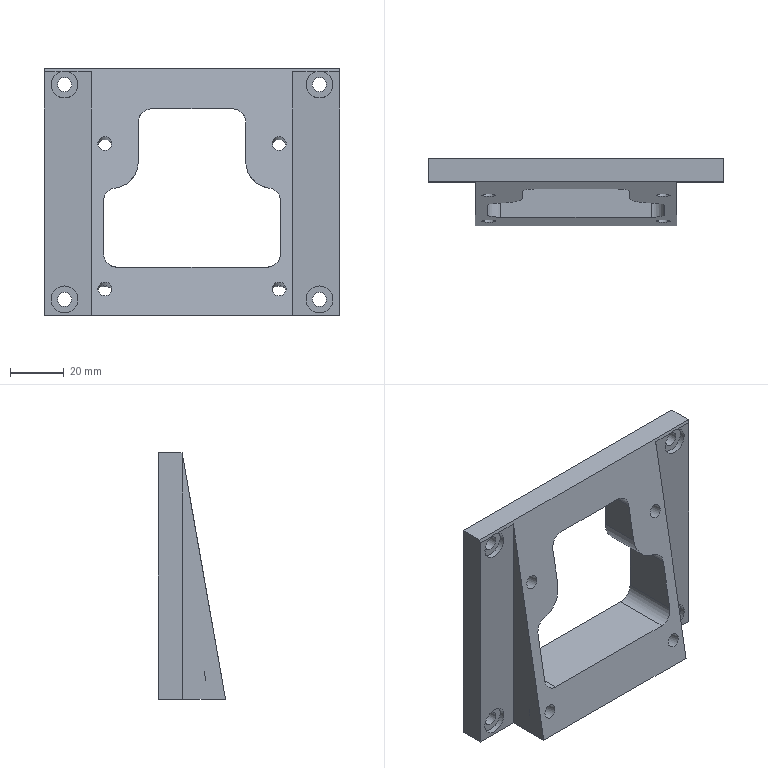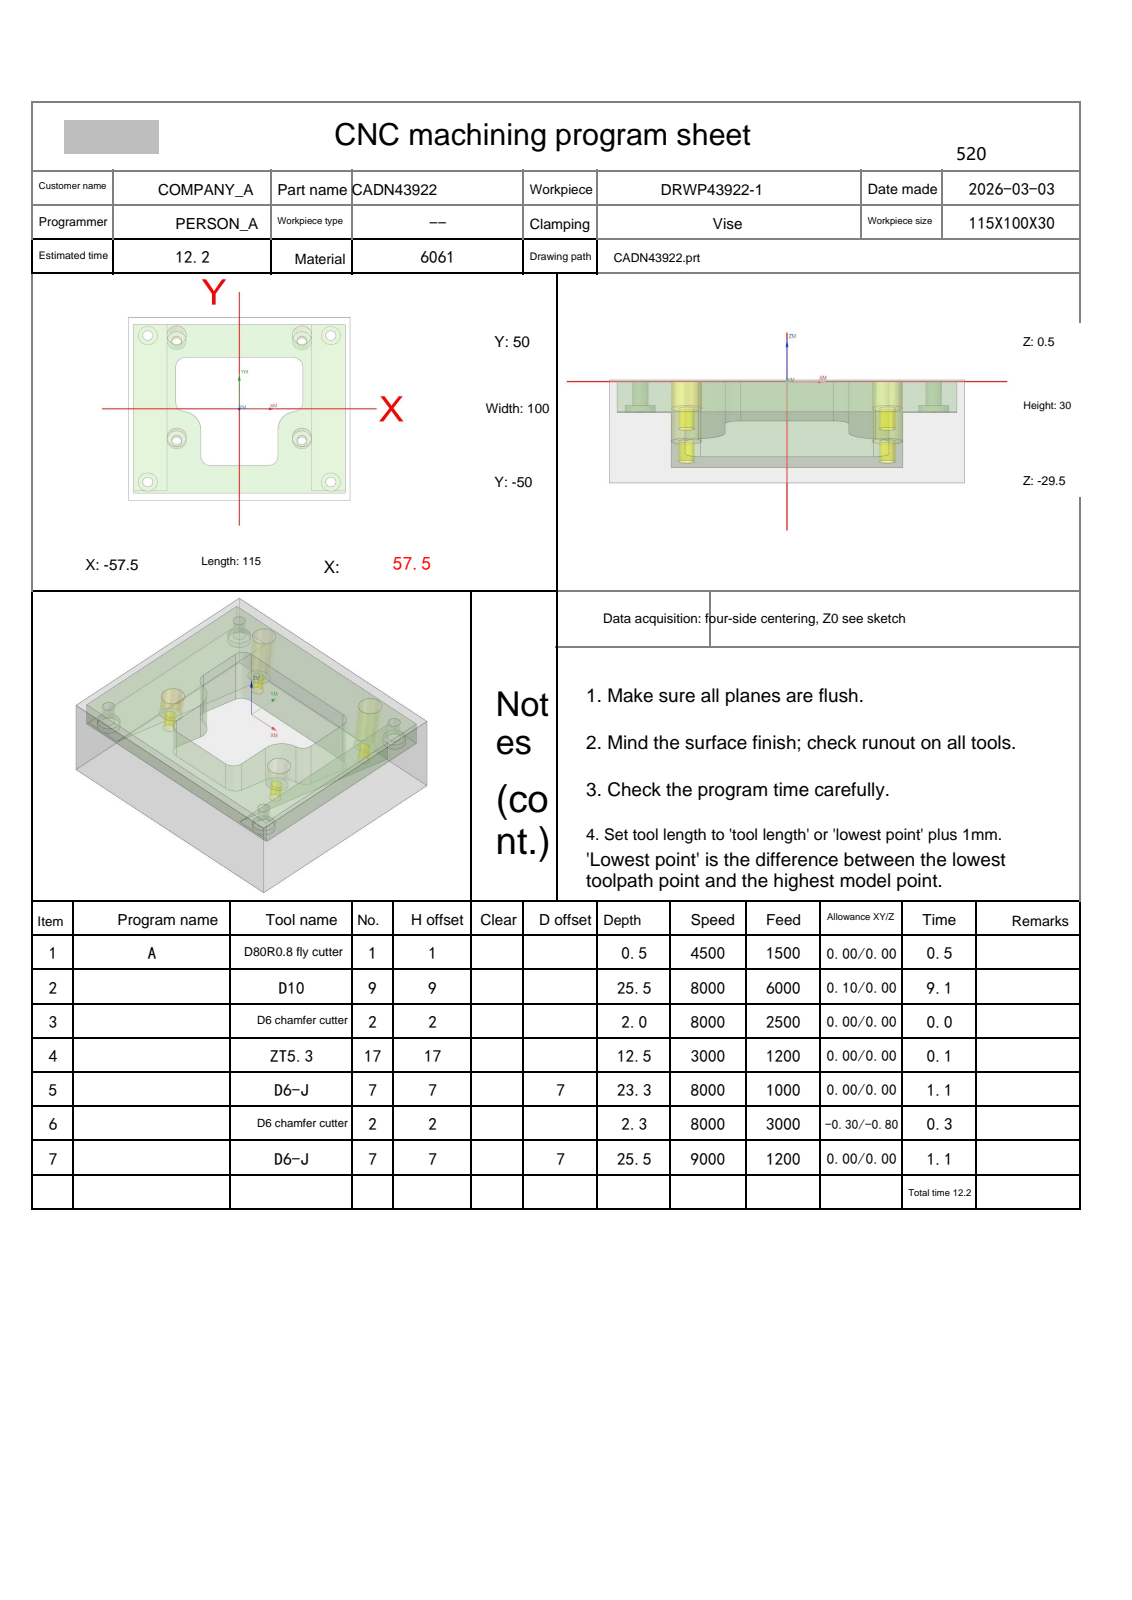NC program | NX | posted by the shop | part box 110 x 25 x 92 mm
Lines 4267 to 4607 of 4607:
N3 T02 M06
(D6 chamfer cutter  D=6. R=0. H=02 ce=0.00 di=0.10)
G00 G90 G54 X47.5 Y40. M03 S8000
G43 H02 Z50.
M08
G98 G81 X47.5 Y40. Z-1.5 R1. F2500.
Y-40.
X-47.5
Y40.
G80
G00 Z50.
G91 G28 Z0.0
M05
M09
G91 G28 Z0.0
M01
N4 T17 M06
(ZT5.3 D=5.3 DR_a=118 H=17)
G00 G90 G54 X47.5 Y40. M03 S3000
G43 H17 Z50.
M08
G98 G83 X47.5 Y40. Z-12. R1. F1200. Q1.5
Y-40.
X-47.5
Y40.
G80
G00 Z50.
G91 G28 Z0.0
M05
M09
G91 G28 Z0.0
M01
N5 T07 M06
(D6-J  D=6. R=0. H=07 ce=0.00 di=0.00)
G00 G90 G54 X29. Y22.801 M03 S8000
G43 H07 Z50.
M08
Z-4.065
G01 Z-4.565 F1000.
G41 D07
Y24.
G03 X28. Y25. I-1. J0.0
G01 X-28.
G03 X-30. Y23. I0.0 J-2.
G01 Y3.5
G03 X-28.267 Y1.518 I2. J0.0
G02 X-17. Y-11.366 I-1.733 J-12.884
G01 Y-26.
G03 X-15. Y-28. I2. J0.0
G01 X15.
G03 X17. Y-26. I0.0 J2.
G01 Y-11.366
G02 X28.267 Y1.518 I13. J0.0
G03 X30. Y3.5 I-.267 J1.982
G01 Y23.
G03 X28. Y25. I-2. J0.0
G01 X27.5
G03 X26.5 Y24. I0.0 J-1.
G01 G40 Y23.8
Z-4.065
G00 X29. Y22.801
Z-8.63
G01 Z-9.13
G41 D07
Y24.
G03 X28. Y25. I-1. J0.0
G01 X-28.
G03 X-30. Y23. I0.0 J-2.
G01 Y3.5
G03 X-28.267 Y1.518 I2. J0.0
G02 X-17. Y-11.366 I-1.733 J-12.884
G01 Y-26.
G03 X-15. Y-28. I2. J0.0
G01 X15.
G03 X17. Y-26. I0.0 J2.
G01 Y-11.366
G02 X28.267 Y1.518 I13. J0.0
G03 X30. Y3.5 I-.267 J1.982
G01 Y23.
G03 X28. Y25. I-2. J0.0
G01 X27.5
G03 X26.5 Y24. I0.0 J-1.
G01 G40 Y23.8
Z-8.63
G00 X29.
Z-13.196
G01 Z-13.696
G41 D07
Y24.
G03 X28. Y25. I-1. J0.0
G01 X-28.
G03 X-30. Y23. I0.0 J-2.
G01 Y3.5
G03 X-28.267 Y1.518 I2. J0.0
G02 X-17. Y-11.366 I-1.733 J-12.884
G01 Y-26.
G03 X-15. Y-28. I2. J0.0
G01 X15.
G03 X17. Y-26. I0.0 J2.
G01 Y-11.366
G02 X28.267 Y1.518 I13. J0.0
G03 X30. Y3.5 I-.267 J1.982
G01 Y23.
G03 X28. Y25. I-2. J0.0
G01 X27.5
G03 X26.5 Y24. I0.0 J-1.
G01 G40 Y23.8
Z-13.196
G00 X29. Y22.801
Z-17.761
G01 Z-18.261
G41 D07
Y24.
G03 X28. Y25. I-1. J0.0
G01 X-28.
G03 X-30. Y23. I0.0 J-2.
G01 Y3.5
G03 X-28.267 Y1.518 I2. J0.0
G02 X-17. Y-11.366 I-1.733 J-12.884
G01 Y-26.
G03 X-15. Y-28. I2. J0.0
G01 X15.
G03 X17. Y-26. I0.0 J2.
G01 Y-11.366
G02 X28.267 Y1.518 I13. J0.0
G03 X30. Y3.5 I-.267 J1.982
G01 Y23.
G03 X28. Y25. I-2. J0.0
G01 X27.5
G03 X26.5 Y24. I0.0 J-1.
G01 G40 Y23.8
Z-17.761
G00 X29. Y22.801
Z-22.326
G01 Z-22.826
G41 D07
Y24.
G03 X28. Y25. I-1. J0.0
G01 X-28.
G03 X-30. Y23. I0.0 J-2.
G01 Y3.5
G03 X-28.267 Y1.518 I2. J0.0
G02 X-17. Y-11.366 I-1.733 J-12.884
G01 Y-26.
G03 X-15. Y-28. I2. J0.0
G01 X15.
G03 X17. Y-26. I0.0 J2.
G01 Y-11.366
G02 X28.267 Y1.518 I13. J0.0
G03 X30. Y3.5 I-.267 J1.982
G01 Y23.
G03 X28. Y25. I-2. J0.0
G01 X27.5
G03 X26.5 Y24. I0.0 J-1.
G01 G40 Y23.8
Z-22.326
G00 Z50.
G91 G28 Z0.0
M05
M09
G91 G28 Z0.0
M01
N6 T02 M06
(D6 chamfer cutter  D=6. R=0. H=02 ce=0.00 di=0.00)
G00 G90 G54 X-57.128 Y-46.25 M03 S8000
G43 H02 Z50.
M08
Z2.085
G01 Z-1.5 F3000.
G03 X-56.828 Y-46.33 I.3 J.52
X-56.308 Y-46.03 I0.0 J.6
G01 X-56.3 Y-46.
Y46.
G02 X-55. Y47.3 I1.3 J0.0
G01 X55.
G02 X56.3 Y46. I0.0 J-1.3
G01 Y-46.
X56.308 Y-46.03
G03 X56.828 Y-46.33 I.52 J.3
X57.128 Y-46.25 I0.0 J.6
G01 Z2.085
G00 Z50.
X.25 Y25.872
Z2.099
G01 Z-1.5
G03 X.33 Y26.172 I-.52 J.3
X.03 Y26.692 I-.6 J0.0
G01 X0.0 Y26.7
X-28.
G03 X-31.7 Y23. I0.0 J-3.7
G01 Y3.5
G03 X-28.493 Y-.167 I3.7 J0.0
G02 X-18.7 Y-11.366 I-1.507 J-11.199
G01 Y-26.
G03 X-15. Y-29.7 I3.7 J0.0
G01 X15.
G03 X18.7 Y-26. I0.0 J3.7
G01 Y-11.366
G02 X28.493 Y-.167 I11.3 J0.0
G03 X31.7 Y3.5 I-.493 J3.667
G01 Y23.
G03 X28. Y26.7 I-3.7 J0.0
G01 X0.0
X-.03 Y26.692
G03 X-.33 Y26.172 I.3 J-.52
X-.25 Y25.872 I.6 J0.0
G01 Z2.099
G00 Z50.
G00 G90 X47.649 Y-39.987 M03 S8000
Z50.
Z-1.3
G01 Z-1.8 F600.
X47.676 Y-39.985
G03 X47.718 Y-39.629 I-1.457 J.355
X47.5 Y-38.85 I-1.5 J0.0
X46.35 Y-40. I0.0 J-1.15
X47.5 Y-41.15 I1.15 J0.0
X48.65 Y-40. I0.0 J1.15
X47.5 Y-38.85 I-1.15 J0.0
X47.282 Y-39.629 I1.282 J-.779
X47.324 Y-39.985 I1.5 J0.0
G01 X47.351 Y-39.987
Z-1.3
G00 Z50.
X47.649 Y40.013
Z-1.3
G01 Z-1.8
X47.676 Y40.015
G03 X47.718 Y40.371 I-1.457 J.355
X47.5 Y41.15 I-1.5 J0.0
X46.35 Y40. I0.0 J-1.15
X47.5 Y38.85 I1.15 J0.0
X48.65 Y40. I0.0 J1.15
X47.5 Y41.15 I-1.15 J0.0
X47.282 Y40.371 I1.282 J-.779
X47.324 Y40.015 I1.5 J0.0
G01 X47.351 Y40.013
Z-1.3
G00 Z50.
X-47.649 Y39.987
Z-1.3
G01 Z-1.8
X-47.676 Y39.985
G03 X-47.718 Y39.629 I1.457 J-.355
X-47.5 Y38.85 I1.5 J0.0
X-46.35 Y40. I0.0 J1.15
X-47.5 Y41.15 I-1.15 J0.0
X-48.65 Y40. I0.0 J-1.15
X-47.5 Y38.85 I1.15 J0.0
X-47.282 Y39.629 I-1.282 J.779
X-47.324 Y39.985 I-1.5 J0.0
G01 X-47.351 Y39.987
Z-1.3
G00 Z50.
X-47.649 Y-40.013
Z-1.3
G01 Z-1.8
X-47.676 Y-40.015
G03 X-47.718 Y-40.371 I1.457 J-.355
X-47.5 Y-41.15 I1.5 J0.0
X-46.35 Y-40. I0.0 J1.15
X-47.5 Y-38.85 I-1.15 J0.0
X-48.65 Y-40. I0.0 J-1.15
X-47.5 Y-41.15 I1.15 J0.0
X-47.282 Y-40.371 I-1.282 J.779
X-47.324 Y-40.015 I-1.5 J0.0
G01 X-47.351 Y-40.013
Z-1.3
G00 Z50.
G91 G28 Z0.0
M05
M09
G91 G28 Z0.0
M01
N7 T07 M06
(D6-J  D=6. R=0. H=07 ce=0.00 di=0.00)
G00 G90 G54 X56.017 Y-50.073 M03 S9000
G43 H07 Z50.
M08
Z-7.833
G01 Z-8.333 F1200.
G41 D07
X55.992 Y-49.875
G03 X55. Y-49. I-.992 J-.125
G01 X-55.
G02 X-58. Y-46. I0.0 J3.
G01 Y46.
G02 X-55. Y49. I3. J0.0
G01 X55.
G02 X58. Y46. I0.0 J-3.
G01 Y-46.
G02 X55. Y-49. I-3. J0.0
G01 X54.5
G03 X53.5 Y-50. I0.0 J-1.
G01 G40 Y-50.2
Z-7.833
G00 Z50.
X56.017 Y-50.073
Z-16.167
G01 Z-16.667
G41 D07
X55.992 Y-49.875
G03 X55. Y-49. I-.992 J-.125
G01 X-55.
G02 X-58. Y-46. I0.0 J3.
G01 Y46.
G02 X-55. Y49. I3. J0.0
G01 X55.
G02 X58. Y46. I0.0 J-3.
G01 Y-46.
G02 X55. Y-49. I-3. J0.0
G01 X54.5
G03 X53.5 Y-50. I0.0 J-1.
G01 G40 Y-50.2
Z-16.167
G00 Z50.
X56.017 Y-50.073
Z-24.5
G01 Z-25.
G41 D07
X55.992 Y-49.875
G03 X55. Y-49. I-.992 J-.125
G01 X-55.
G02 X-58. Y-46. I0.0 J3.
G01 Y46.
G02 X-55. Y49. I3. J0.0
G01 X55.
G02 X58. Y46. I0.0 J-3.
G01 Y-46.
G02 X55. Y-49. I-3. J0.0
G01 X54.5
G03 X53.5 Y-50. I0.0 J-1.
G01 G40 Y-50.2
Z-24.5
G00 Z50.
M05
M09
G91 G28 Z0.0
G91 G28 Y0.0
M30
%